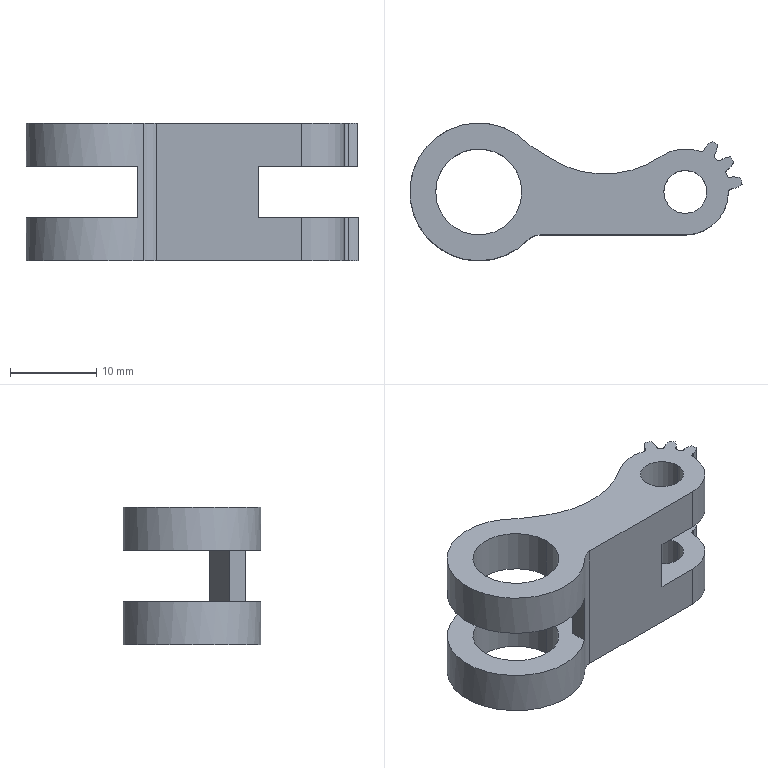Part | SolidWorks | features HoleWzd 4, ICE 4, Fillet 2, RefSurface 2, ThickenCut 2, Extrusion 1 | 1 solid | 51 faces | box 38.582 x 16 x 16 mm | volume 3069 mm3 | cylinder 28 | plane 15 | spline 8 | commonest cylinder face diameters 10 x8 13.28 x6 1 x4 5 x4 4 x3 23.228 x2